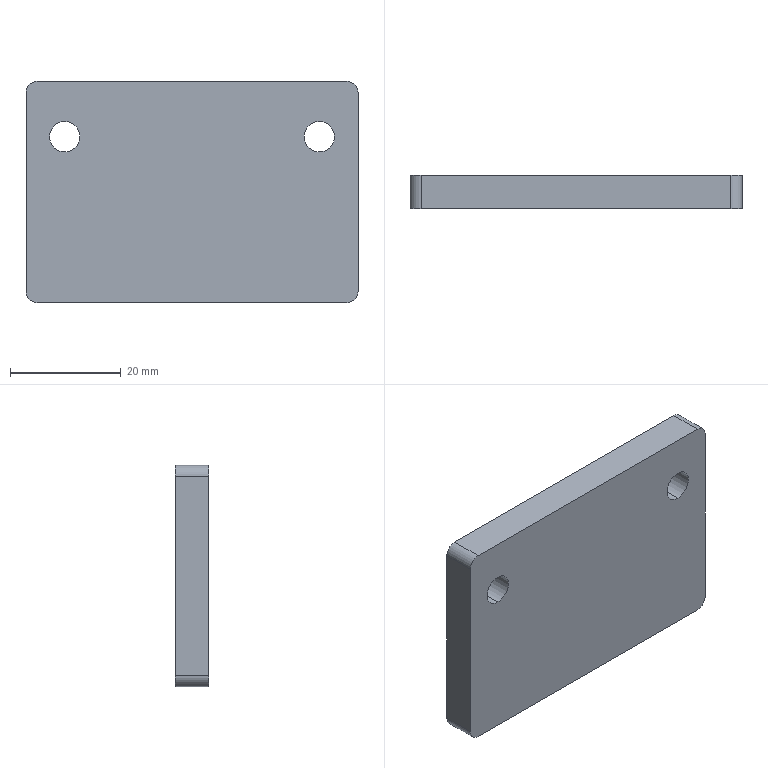Part | SolidWorks | features BaseBody 1 | 1 solid | 14 faces | box 60 x 6 x 40 mm | volume 14094 mm3 | cylinder 8 | plane 6 | commonest cylinder face diameters 4 x4 5.5 x4
STEP:
#1=CARTESIAN_POINT('',(23.,6.,12.75));
#2=VERTEX_POINT('',#1);
#3=CARTESIAN_POINT('',(23.,6.,7.25));
#4=VERTEX_POINT('',#3);
#5=CARTESIAN_POINT('',(23.,6.,10.));
#6=DIRECTION('',(0.,-1.,0.));
#7=DIRECTION('',(0.,0.,-1.));
#8=AXIS2_PLACEMENT_3D('',#5,#6,#7);
#9=CIRCLE('',#8,2.75);
#10=EDGE_CURVE('',#2,#4,#9,.T.);
#11=ORIENTED_EDGE('',*,*,#10,.F.);
#12=CARTESIAN_POINT('',(23.,0.,12.75));
#13=VERTEX_POINT('',#12);
#14=CARTESIAN_POINT('',(23.,6.,12.75));
#15=DIRECTION('',(0.,-1.,0.));
#16=VECTOR('',#15,1000.);
#17=LINE('',#14,#16);
#18=EDGE_CURVE('',#2,#13,#17,.T.);
#19=ORIENTED_EDGE('',*,*,#18,.T.);
#20=CARTESIAN_POINT('',(23.,0.,7.25));
#21=VERTEX_POINT('',#20);
#22=CARTESIAN_POINT('',(23.,0.,10.));
#23=DIRECTION('',(0.,1.,0.));
#24=DIRECTION('',(0.,0.,-1.));
#25=AXIS2_PLACEMENT_3D('',#22,#23,#24);
#26=CIRCLE('',#25,2.75);
#27=EDGE_CURVE('',#21,#13,#26,.T.);
#28=ORIENTED_EDGE('',*,*,#27,.F.);
#29=CARTESIAN_POINT('',(23.,6.,7.25));
#30=DIRECTION('',(0.,-1.,0.));
#31=VECTOR('',#30,1000.);
#32=LINE('',#29,#31);
#33=EDGE_CURVE('',#4,#21,#32,.T.);
#34=ORIENTED_EDGE('',*,*,#33,.F.);
#35=EDGE_LOOP('',(#11,#19,#28,#34));
#36=FACE_OUTER_BOUND('',#35,.T.);
#37=CARTESIAN_POINT('',(23.,6.,10.));
#38=DIRECTION('',(0.,-1.,0.));
#39=DIRECTION('',(0.,0.,-1.));
#40=AXIS2_PLACEMENT_3D('',#37,#38,#39);
#41=CYLINDRICAL_SURFACE('',#40,2.75);
#42=ADVANCED_FACE('',(#36),#41,.F.);
#43=CARTESIAN_POINT('',(-23.,6.,12.75));
#44=VERTEX_POINT('',#43);
#45=CARTESIAN_POINT('',(-23.,6.,7.25));
#46=VERTEX_POINT('',#45);
#47=CARTESIAN_POINT('',(-23.,6.,10.));
#48=DIRECTION('',(0.,-1.,0.));
#49=DIRECTION('',(0.,0.,-1.));
#50=AXIS2_PLACEMENT_3D('',#47,#48,#49);
#51=CIRCLE('',#50,2.75);
#52=EDGE_CURVE('',#44,#46,#51,.T.);
#53=ORIENTED_EDGE('',*,*,#52,.F.);
#54=CARTESIAN_POINT('',(-23.,0.,12.75));
#55=VERTEX_POINT('',#54);
#56=CARTESIAN_POINT('',(-23.,6.,12.75));
#57=DIRECTION('',(0.,-1.,0.));
#58=VECTOR('',#57,1000.);
#59=LINE('',#56,#58);
#60=EDGE_CURVE('',#44,#55,#59,.T.);
#61=ORIENTED_EDGE('',*,*,#60,.T.);
#62=CARTESIAN_POINT('',(-23.,0.,7.25));
#63=VERTEX_POINT('',#62);
#64=CARTESIAN_POINT('',(-23.,0.,10.));
#65=DIRECTION('',(0.,1.,0.));
#66=DIRECTION('',(0.,0.,-1.));
#67=AXIS2_PLACEMENT_3D('',#64,#65,#66);
#68=CIRCLE('',#67,2.75);
#69=EDGE_CURVE('',#63,#55,#68,.T.);
#70=ORIENTED_EDGE('',*,*,#69,.F.);
#71=CARTESIAN_POINT('',(-23.,6.,7.25));
#72=DIRECTION('',(0.,-1.,0.));
#73=VECTOR('',#72,1000.);
#74=LINE('',#71,#73);
#75=EDGE_CURVE('',#46,#63,#74,.T.);
#76=ORIENTED_EDGE('',*,*,#75,.F.);
#77=EDGE_LOOP('',(#53,#61,#70,#76));
#78=FACE_OUTER_BOUND('',#77,.T.);
#79=CARTESIAN_POINT('',(-23.,6.,10.));
#80=DIRECTION('',(0.,-1.,0.));
#81=DIRECTION('',(0.,0.,-1.));
#82=AXIS2_PLACEMENT_3D('',#79,#80,#81);
#83=CYLINDRICAL_SURFACE('',#82,2.75);
#84=ADVANCED_FACE('',(#78),#83,.F.);
#85=CARTESIAN_POINT('',(23.,6.,10.));
#86=DIRECTION('',(0.,-1.,0.));
#87=DIRECTION('',(0.,0.,-1.));
#88=AXIS2_PLACEMENT_3D('',#85,#86,#87);
#89=CIRCLE('',#88,2.75);
#90=EDGE_CURVE('',#4,#2,#89,.T.);
#91=ORIENTED_EDGE('',*,*,#90,.T.);
#92=ORIENTED_EDGE('',*,*,#10,.T.);
#93=EDGE_LOOP('',(#91,#92));
#94=FACE_BOUND('',#93,.T.);
#95=CARTESIAN_POINT('',(-30.,6.,-18.));
#96=VERTEX_POINT('',#95);
#97=CARTESIAN_POINT('',(-30.,6.,18.));
#98=VERTEX_POINT('',#97);
#99=CARTESIAN_POINT('',(-30.,6.,0.));
#100=DIRECTION('',(0.,0.,1.));
#101=VECTOR('',#100,1000.);
#102=LINE('',#99,#101);
#103=EDGE_CURVE('',#96,#98,#102,.T.);
#104=ORIENTED_EDGE('',*,*,#103,.T.);
#105=CARTESIAN_POINT('',(-28.,6.,20.));
#106=VERTEX_POINT('',#105);
#107=CARTESIAN_POINT('',(-28.,6.,18.));
#108=DIRECTION('',(0.,1.,0.));
#109=DIRECTION('',(0.,0.,-1.));
#110=AXIS2_PLACEMENT_3D('',#107,#108,#109);
#111=CIRCLE('',#110,2.);
#112=EDGE_CURVE('',#98,#106,#111,.T.);
#113=ORIENTED_EDGE('',*,*,#112,.T.);
#114=CARTESIAN_POINT('',(28.,6.,20.));
#115=VERTEX_POINT('',#114);
#116=CARTESIAN_POINT('',(0.,6.,20.));
#117=DIRECTION('',(1.,0.,0.));
#118=VECTOR('',#117,1000.);
#119=LINE('',#116,#118);
#120=EDGE_CURVE('',#106,#115,#119,.T.);
#121=ORIENTED_EDGE('',*,*,#120,.T.);
#122=CARTESIAN_POINT('',(30.,6.,18.));
#123=VERTEX_POINT('',#122);
#124=CARTESIAN_POINT('',(28.,6.,18.));
#125=DIRECTION('',(0.,1.,0.));
#126=DIRECTION('',(0.,0.,-1.));
#127=AXIS2_PLACEMENT_3D('',#124,#125,#126);
#128=CIRCLE('',#127,2.);
#129=EDGE_CURVE('',#115,#123,#128,.T.);
#130=ORIENTED_EDGE('',*,*,#129,.T.);
#131=CARTESIAN_POINT('',(30.,6.,-18.));
#132=VERTEX_POINT('',#131);
#133=CARTESIAN_POINT('',(30.,6.,0.));
#134=DIRECTION('',(0.,0.,-1.));
#135=VECTOR('',#134,1000.);
#136=LINE('',#133,#135);
#137=EDGE_CURVE('',#123,#132,#136,.T.);
#138=ORIENTED_EDGE('',*,*,#137,.T.);
#139=CARTESIAN_POINT('',(28.,6.,-20.));
#140=VERTEX_POINT('',#139);
#141=CARTESIAN_POINT('',(28.,6.,-18.));
#142=DIRECTION('',(0.,1.,0.));
#143=DIRECTION('',(0.,0.,-1.));
#144=AXIS2_PLACEMENT_3D('',#141,#142,#143);
#145=CIRCLE('',#144,2.);
#146=EDGE_CURVE('',#132,#140,#145,.T.);
#147=ORIENTED_EDGE('',*,*,#146,.T.);
#148=CARTESIAN_POINT('',(-28.,6.,-20.));
#149=VERTEX_POINT('',#148);
#150=CARTESIAN_POINT('',(0.,6.,-20.));
#151=DIRECTION('',(-1.,0.,0.));
#152=VECTOR('',#151,1000.);
#153=LINE('',#150,#152);
#154=EDGE_CURVE('',#140,#149,#153,.T.);
#155=ORIENTED_EDGE('',*,*,#154,.T.);
#156=CARTESIAN_POINT('',(-28.,6.,-18.));
#157=DIRECTION('',(0.,1.,0.));
#158=DIRECTION('',(0.,0.,-1.));
#159=AXIS2_PLACEMENT_3D('',#156,#157,#158);
#160=CIRCLE('',#159,2.);
#161=EDGE_CURVE('',#149,#96,#160,.T.);
#162=ORIENTED_EDGE('',*,*,#161,.T.);
#163=EDGE_LOOP('',(#104,#113,#121,#130,#138,#147,#155,#162));
#164=FACE_OUTER_BOUND('',#163,.T.);
#165=CARTESIAN_POINT('',(-23.,6.,10.));
#166=DIRECTION('',(0.,-1.,0.));
#167=DIRECTION('',(0.,0.,-1.));
#168=AXIS2_PLACEMENT_3D('',#165,#166,#167);
#169=CIRCLE('',#168,2.75);
#170=EDGE_CURVE('',#46,#44,#169,.T.);
#171=ORIENTED_EDGE('',*,*,#170,.T.);
#172=ORIENTED_EDGE('',*,*,#52,.T.);
#173=EDGE_LOOP('',(#171,#172));
#174=FACE_BOUND('',#173,.T.);
#175=CARTESIAN_POINT('',(0.,6.,0.));
#176=DIRECTION('',(0.,1.,0.));
#177=DIRECTION('',(0.,0.,1.));
#178=AXIS2_PLACEMENT_3D('',#175,#176,#177);
#179=PLANE('',#178);
#180=ADVANCED_FACE('',(#94,#164,#174),#179,.T.);
#181=ORIENTED_EDGE('',*,*,#18,.F.);
#182=ORIENTED_EDGE('',*,*,#90,.F.);
#183=ORIENTED_EDGE('',*,*,#33,.T.);
#184=CARTESIAN_POINT('',(23.,0.,10.));
#185=DIRECTION('',(0.,1.,0.));
#186=DIRECTION('',(0.,0.,-1.));
#187=AXIS2_PLACEMENT_3D('',#184,#185,#186);
#188=CIRCLE('',#187,2.75);
#189=EDGE_CURVE('',#13,#21,#188,.T.);
#190=ORIENTED_EDGE('',*,*,#189,.F.);
#191=EDGE_LOOP('',(#181,#182,#183,#190));
#192=FACE_OUTER_BOUND('',#191,.T.);
#193=CARTESIAN_POINT('',(23.,6.,10.));
#194=DIRECTION('',(0.,-1.,0.));
#195=DIRECTION('',(0.,0.,-1.));
#196=AXIS2_PLACEMENT_3D('',#193,#194,#195);
#197=CYLINDRICAL_SURFACE('',#196,2.75);
#198=ADVANCED_FACE('',(#192),#197,.F.);
#199=CARTESIAN_POINT('',(-30.,0.,18.));
#200=VERTEX_POINT('',#199);
#201=CARTESIAN_POINT('',(-28.,0.,20.));
#202=VERTEX_POINT('',#201);
#203=CARTESIAN_POINT('',(-28.,0.,18.));
#204=DIRECTION('',(0.,1.,0.));
#205=DIRECTION('',(0.,0.,-1.));
#206=AXIS2_PLACEMENT_3D('',#203,#204,#205);
#207=CIRCLE('',#206,2.);
#208=EDGE_CURVE('',#200,#202,#207,.T.);
#209=ORIENTED_EDGE('',*,*,#208,.T.);
#210=CARTESIAN_POINT('',(-28.,6.,20.));
#211=DIRECTION('',(0.,1.,0.));
#212=VECTOR('',#211,1000.);
#213=LINE('',#210,#212);
#214=EDGE_CURVE('',#202,#106,#213,.T.);
#215=ORIENTED_EDGE('',*,*,#214,.T.);
#216=ORIENTED_EDGE('',*,*,#112,.F.);
#217=CARTESIAN_POINT('',(-30.,6.,18.));
#218=DIRECTION('',(0.,-1.,0.));
#219=VECTOR('',#218,1000.);
#220=LINE('',#217,#219);
#221=EDGE_CURVE('',#98,#200,#220,.T.);
#222=ORIENTED_EDGE('',*,*,#221,.T.);
#223=EDGE_LOOP('',(#209,#215,#216,#222));
#224=FACE_OUTER_BOUND('',#223,.T.);
#225=CARTESIAN_POINT('',(-28.,6.,18.));
#226=DIRECTION('',(0.,-1.,0.));
#227=DIRECTION('',(0.,0.,-1.));
#228=AXIS2_PLACEMENT_3D('',#225,#226,#227);
#229=CYLINDRICAL_SURFACE('',#228,2.);
#230=ADVANCED_FACE('',(#224),#229,.T.);
#231=CARTESIAN_POINT('',(-30.,0.,-18.));
#232=VERTEX_POINT('',#231);
#233=CARTESIAN_POINT('',(-30.,6.,-18.));
#234=DIRECTION('',(0.,1.,0.));
#235=VECTOR('',#234,1000.);
#236=LINE('',#233,#235);
#237=EDGE_CURVE('',#232,#96,#236,.T.);
#238=ORIENTED_EDGE('',*,*,#237,.F.);
#239=CARTESIAN_POINT('',(-30.,0.,20.));
#240=DIRECTION('',(0.,0.,-1.));
#241=VECTOR('',#240,1000.);
#242=LINE('',#239,#241);
#243=EDGE_CURVE('',#200,#232,#242,.T.);
#244=ORIENTED_EDGE('',*,*,#243,.F.);
#245=ORIENTED_EDGE('',*,*,#221,.F.);
#246=ORIENTED_EDGE('',*,*,#103,.F.);
#247=EDGE_LOOP('',(#238,#244,#245,#246));
#248=FACE_OUTER_BOUND('',#247,.T.);
#249=CARTESIAN_POINT('',(-30.,6.,20.));
#250=DIRECTION('',(1.,0.,0.));
#251=DIRECTION('',(0.,0.,-1.));
#252=AXIS2_PLACEMENT_3D('',#249,#250,#251);
#253=PLANE('',#252);
#254=ADVANCED_FACE('',(#248),#253,.F.);
#255=CARTESIAN_POINT('',(-28.,0.,-20.));
#256=VERTEX_POINT('',#255);
#257=CARTESIAN_POINT('',(-28.,0.,-18.));
#258=DIRECTION('',(0.,1.,0.));
#259=DIRECTION('',(0.,0.,-1.));
#260=AXIS2_PLACEMENT_3D('',#257,#258,#259);
#261=CIRCLE('',#260,2.);
#262=EDGE_CURVE('',#256,#232,#261,.T.);
#263=ORIENTED_EDGE('',*,*,#262,.T.);
#264=ORIENTED_EDGE('',*,*,#237,.T.);
#265=ORIENTED_EDGE('',*,*,#161,.F.);
#266=CARTESIAN_POINT('',(-28.,6.,-20.));
#267=DIRECTION('',(0.,-1.,0.));
#268=VECTOR('',#267,1000.);
#269=LINE('',#266,#268);
#270=EDGE_CURVE('',#149,#256,#269,.T.);
#271=ORIENTED_EDGE('',*,*,#270,.T.);
#272=EDGE_LOOP('',(#263,#264,#265,#271));
#273=FACE_OUTER_BOUND('',#272,.T.);
#274=CARTESIAN_POINT('',(-28.,6.,-18.));
#275=DIRECTION('',(0.,-1.,0.));
#276=DIRECTION('',(0.,0.,-1.));
#277=AXIS2_PLACEMENT_3D('',#274,#275,#276);
#278=CYLINDRICAL_SURFACE('',#277,2.);
#279=ADVANCED_FACE('',(#273),#278,.T.);
#280=CARTESIAN_POINT('',(28.,0.,-20.));
#281=VERTEX_POINT('',#280);
#282=CARTESIAN_POINT('',(28.,6.,-20.));
#283=DIRECTION('',(0.,1.,0.));
#284=VECTOR('',#283,1000.);
#285=LINE('',#282,#284);
#286=EDGE_CURVE('',#281,#140,#285,.T.);
#287=ORIENTED_EDGE('',*,*,#286,.F.);
#288=CARTESIAN_POINT('',(30.,0.,-20.));
#289=DIRECTION('',(1.,0.,0.));
#290=VECTOR('',#289,1000.);
#291=LINE('',#288,#290);
#292=EDGE_CURVE('',#256,#281,#291,.T.);
#293=ORIENTED_EDGE('',*,*,#292,.F.);
#294=ORIENTED_EDGE('',*,*,#270,.F.);
#295=ORIENTED_EDGE('',*,*,#154,.F.);
#296=EDGE_LOOP('',(#287,#293,#294,#295));
#297=FACE_OUTER_BOUND('',#296,.T.);
#298=CARTESIAN_POINT('',(30.,6.,-20.));
#299=DIRECTION('',(0.,0.,1.));
#300=DIRECTION('',(1.,0.,0.));
#301=AXIS2_PLACEMENT_3D('',#298,#299,#300);
#302=PLANE('',#301);
#303=ADVANCED_FACE('',(#297),#302,.F.);
#304=CARTESIAN_POINT('',(30.,0.,-18.));
#305=VERTEX_POINT('',#304);
#306=CARTESIAN_POINT('',(28.,0.,-18.));
#307=DIRECTION('',(0.,1.,0.));
#308=DIRECTION('',(0.,0.,-1.));
#309=AXIS2_PLACEMENT_3D('',#306,#307,#308);
#310=CIRCLE('',#309,2.);
#311=EDGE_CURVE('',#305,#281,#310,.T.);
#312=ORIENTED_EDGE('',*,*,#311,.T.);
#313=ORIENTED_EDGE('',*,*,#286,.T.);
#314=ORIENTED_EDGE('',*,*,#146,.F.);
#315=CARTESIAN_POINT('',(30.,6.,-18.));
#316=DIRECTION('',(0.,-1.,0.));
#317=VECTOR('',#316,1000.);
#318=LINE('',#315,#317);
#319=EDGE_CURVE('',#132,#305,#318,.T.);
#320=ORIENTED_EDGE('',*,*,#319,.T.);
#321=EDGE_LOOP('',(#312,#313,#314,#320));
#322=FACE_OUTER_BOUND('',#321,.T.);
#323=CARTESIAN_POINT('',(28.,6.,-18.));
#324=DIRECTION('',(0.,-1.,0.));
#325=DIRECTION('',(0.,0.,-1.));
#326=AXIS2_PLACEMENT_3D('',#323,#324,#325);
#327=CYLINDRICAL_SURFACE('',#326,2.);
#328=ADVANCED_FACE('',(#322),#327,.T.);
#329=CARTESIAN_POINT('',(30.,0.,18.));
#330=VERTEX_POINT('',#329);
#331=CARTESIAN_POINT('',(30.,6.,18.));
#332=DIRECTION('',(0.,1.,0.));
#333=VECTOR('',#332,1000.);
#334=LINE('',#331,#333);
#335=EDGE_CURVE('',#330,#123,#334,.T.);
#336=ORIENTED_EDGE('',*,*,#335,.F.);
#337=CARTESIAN_POINT('',(30.,0.,20.));
#338=DIRECTION('',(0.,0.,1.));
#339=VECTOR('',#338,1000.);
#340=LINE('',#337,#339);
#341=EDGE_CURVE('',#305,#330,#340,.T.);
#342=ORIENTED_EDGE('',*,*,#341,.F.);
#343=ORIENTED_EDGE('',*,*,#319,.F.);
#344=ORIENTED_EDGE('',*,*,#137,.F.);
#345=EDGE_LOOP('',(#336,#342,#343,#344));
#346=FACE_OUTER_BOUND('',#345,.T.);
#347=CARTESIAN_POINT('',(30.,6.,20.));
#348=DIRECTION('',(-1.,0.,0.));
#349=DIRECTION('',(0.,0.,1.));
#350=AXIS2_PLACEMENT_3D('',#347,#348,#349);
#351=PLANE('',#350);
#352=ADVANCED_FACE('',(#346),#351,.F.);
#353=CARTESIAN_POINT('',(28.,0.,20.));
#354=VERTEX_POINT('',#353);
#355=CARTESIAN_POINT('',(28.,0.,18.));
#356=DIRECTION('',(0.,1.,0.));
#357=DIRECTION('',(0.,0.,-1.));
#358=AXIS2_PLACEMENT_3D('',#355,#356,#357);
#359=CIRCLE('',#358,2.);
#360=EDGE_CURVE('',#354,#330,#359,.T.);
#361=ORIENTED_EDGE('',*,*,#360,.T.);
#362=ORIENTED_EDGE('',*,*,#335,.T.);
#363=ORIENTED_EDGE('',*,*,#129,.F.);
#364=CARTESIAN_POINT('',(28.,6.,20.));
#365=DIRECTION('',(0.,-1.,0.));
#366=VECTOR('',#365,1000.);
#367=LINE('',#364,#366);
#368=EDGE_CURVE('',#115,#354,#367,.T.);
#369=ORIENTED_EDGE('',*,*,#368,.T.);
#370=EDGE_LOOP('',(#361,#362,#363,#369));
#371=FACE_OUTER_BOUND('',#370,.T.);
#372=CARTESIAN_POINT('',(28.,6.,18.));
#373=DIRECTION('',(0.,-1.,0.));
#374=DIRECTION('',(0.,0.,-1.));
#375=AXIS2_PLACEMENT_3D('',#372,#373,#374);
#376=CYLINDRICAL_SURFACE('',#375,2.);
#377=ADVANCED_FACE('',(#371),#376,.T.);
#378=ORIENTED_EDGE('',*,*,#368,.F.);
#379=ORIENTED_EDGE('',*,*,#120,.F.);
#380=ORIENTED_EDGE('',*,*,#214,.F.);
#381=CARTESIAN_POINT('',(30.,0.,20.));
#382=DIRECTION('',(-1.,0.,0.));
#383=VECTOR('',#382,1000.);
#384=LINE('',#381,#383);
#385=EDGE_CURVE('',#354,#202,#384,.T.);
#386=ORIENTED_EDGE('',*,*,#385,.F.);
#387=EDGE_LOOP('',(#378,#379,#380,#386));
#388=FACE_OUTER_BOUND('',#387,.T.);
#389=CARTESIAN_POINT('',(30.,6.,20.));
#390=DIRECTION('',(0.,0.,-1.));
#391=DIRECTION('',(-1.,0.,0.));
#392=AXIS2_PLACEMENT_3D('',#389,#390,#391);
#393=PLANE('',#392);
#394=ADVANCED_FACE('',(#388),#393,.F.);
#395=ORIENTED_EDGE('',*,*,#60,.F.);
#396=ORIENTED_EDGE('',*,*,#170,.F.);
#397=ORIENTED_EDGE('',*,*,#75,.T.);
#398=CARTESIAN_POINT('',(-23.,0.,10.));
#399=DIRECTION('',(0.,1.,0.));
#400=DIRECTION('',(0.,0.,-1.));
#401=AXIS2_PLACEMENT_3D('',#398,#399,#400);
#402=CIRCLE('',#401,2.75);
#403=EDGE_CURVE('',#55,#63,#402,.T.);
#404=ORIENTED_EDGE('',*,*,#403,.F.);
#405=EDGE_LOOP('',(#395,#396,#397,#404));
#406=FACE_OUTER_BOUND('',#405,.T.);
#407=CARTESIAN_POINT('',(-23.,6.,10.));
#408=DIRECTION('',(0.,-1.,0.));
#409=DIRECTION('',(0.,0.,-1.));
#410=AXIS2_PLACEMENT_3D('',#407,#408,#409);
#411=CYLINDRICAL_SURFACE('',#410,2.75);
#412=ADVANCED_FACE('',(#406),#411,.F.);
#413=ORIENTED_EDGE('',*,*,#27,.T.);
#414=ORIENTED_EDGE('',*,*,#189,.T.);
#415=EDGE_LOOP('',(#413,#414));
#416=FACE_BOUND('',#415,.T.);
#417=ORIENTED_EDGE('',*,*,#69,.T.);
#418=ORIENTED_EDGE('',*,*,#403,.T.);
#419=EDGE_LOOP('',(#417,#418));
#420=FACE_BOUND('',#419,.T.);
#421=ORIENTED_EDGE('',*,*,#360,.F.);
#422=ORIENTED_EDGE('',*,*,#385,.T.);
#423=ORIENTED_EDGE('',*,*,#208,.F.);
#424=ORIENTED_EDGE('',*,*,#243,.T.);
#425=ORIENTED_EDGE('',*,*,#262,.F.);
#426=ORIENTED_EDGE('',*,*,#292,.T.);
#427=ORIENTED_EDGE('',*,*,#311,.F.);
#428=ORIENTED_EDGE('',*,*,#341,.T.);
#429=EDGE_LOOP('',(#421,#422,#423,#424,#425,#426,#427,#428));
#430=FACE_OUTER_BOUND('',#429,.T.);
#431=CARTESIAN_POINT('',(0.,0.,0.));
#432=DIRECTION('',(0.,1.,0.));
#433=DIRECTION('',(0.,0.,1.));
#434=AXIS2_PLACEMENT_3D('',#431,#432,#433);
#435=PLANE('',#434);
#436=ADVANCED_FACE('',(#416,#420,#430),#435,.F.);
#437=CLOSED_SHELL('',(#42,#84,#180,#198,#230,#254,#279,#303,#328,#352,#377,#394,#412,#436));
#438=MANIFOLD_SOLID_BREP('',#437);
#439=CARTESIAN_POINT('',(0.,0.,0.));
#440=DIRECTION('',(0.,0.,1.));
#441=DIRECTION('',(1.,0.,0.));
#442=AXIS2_PLACEMENT_3D('',#439,#440,#441);
#443=(LENGTH_UNIT()NAMED_UNIT(*)SI_UNIT(.MILLI.,.METRE.));
#444=UNCERTAINTY_MEASURE_WITH_UNIT(LENGTH_MEASURE(0.00001),#443,'','');
#445=(NAMED_UNIT(*)PLANE_ANGLE_UNIT()SI_UNIT($,.RADIAN.));
#446=(NAMED_UNIT(*)SI_UNIT($,.STERADIAN.)SOLID_ANGLE_UNIT());
#447=(GEOMETRIC_REPRESENTATION_CONTEXT(3)GLOBAL_UNCERTAINTY_ASSIGNED_CONTEXT((#444))GLOBAL_UNIT_ASSIGNED_CONTEXT((#443,#445,#446))REPRESENTATION_CONTEXT('',''));
#448=ADVANCED_BREP_SHAPE_REPRESENTATION('',(#438,#442),#447);